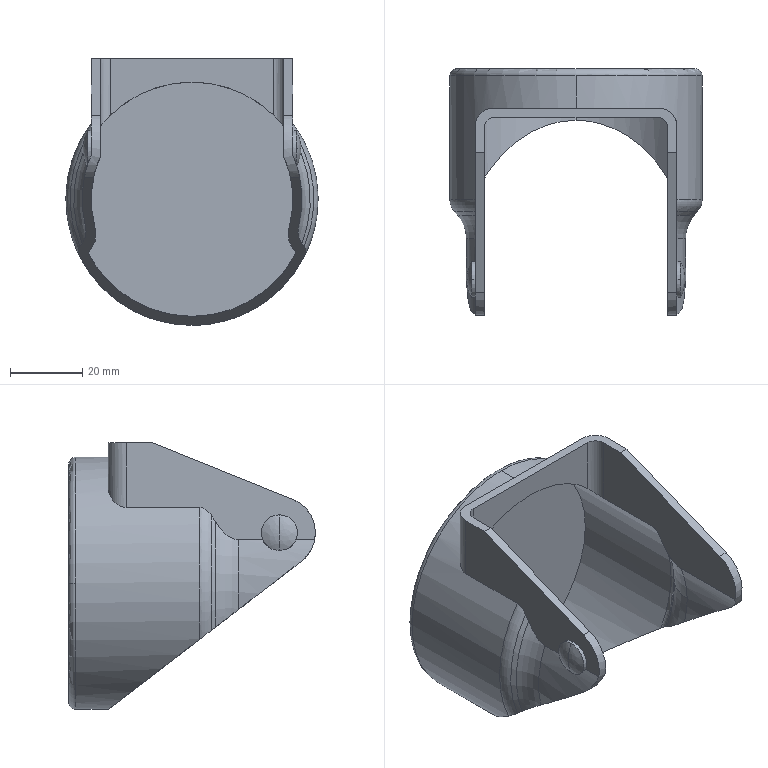Part | SolidWorks | features BaseBody 1 | 1 solid | 50 faces | box 70 x 68.5 x 74 mm | volume 29160 mm3 | cylinder 18 | torus 12 | plane 12 | spline 4 | cone 4 | commonest cylinder face diameters 10 x6 6 x2 20 x2 56 x2 61 x2 65 x2